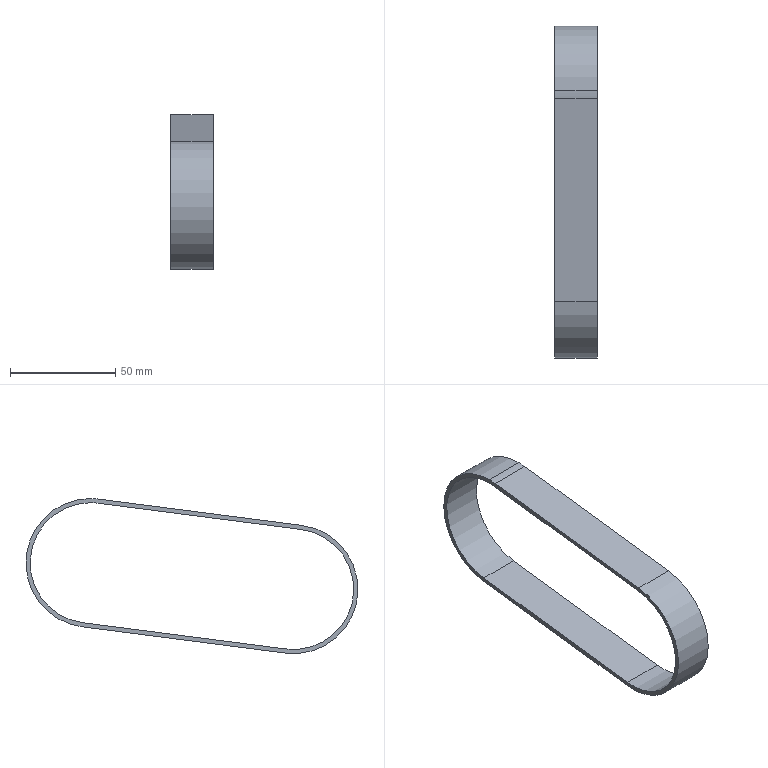Part | SolidWorks | features BaseBody 1 | 1 solid | 12 faces | box 20 x 157.99 x 73.8 mm | volume 15251 mm3 | cylinder 6 | plane 6 | commonest cylinder face diameters 57.3 x3 61.3 x3
STEP:
#1=CARTESIAN_POINT('',(20.,3.673,-28.414));
#2=VERTEX_POINT('',#1);
#3=CARTESIAN_POINT('',(20.,0.,28.65));
#4=VERTEX_POINT('',#3);
#5=CARTESIAN_POINT('',(20.,0.,0.));
#6=DIRECTION('',(1.,0.,0.));
#7=DIRECTION('',(0.,0.,-1.));
#8=AXIS2_PLACEMENT_3D('',#5,#6,#7);
#9=CIRCLE('',#8,28.65);
#10=EDGE_CURVE('',#2,#4,#9,.T.);
#11=ORIENTED_EDGE('',*,*,#10,.T.);
#12=CARTESIAN_POINT('',(0.,0.,28.65));
#13=VERTEX_POINT('',#12);
#14=CARTESIAN_POINT('',(20.,0.,28.65));
#15=DIRECTION('',(-1.,0.,0.));
#16=VECTOR('',#15,1000.);
#17=LINE('',#14,#16);
#18=EDGE_CURVE('',#4,#13,#17,.T.);
#19=ORIENTED_EDGE('',*,*,#18,.T.);
#20=CARTESIAN_POINT('',(0.,3.673,-28.414));
#21=VERTEX_POINT('',#20);
#22=CARTESIAN_POINT('',(0.,0.,0.));
#23=DIRECTION('',(1.,0.,0.));
#24=DIRECTION('',(0.,0.,-1.));
#25=AXIS2_PLACEMENT_3D('',#22,#23,#24);
#26=CIRCLE('',#25,28.65);
#27=EDGE_CURVE('',#21,#13,#26,.T.);
#28=ORIENTED_EDGE('',*,*,#27,.F.);
#29=CARTESIAN_POINT('',(20.,3.673,-28.414));
#30=DIRECTION('',(-1.,0.,0.));
#31=VECTOR('',#30,1000.);
#32=LINE('',#29,#31);
#33=EDGE_CURVE('',#2,#21,#32,.T.);
#34=ORIENTED_EDGE('',*,*,#33,.F.);
#35=EDGE_LOOP('',(#11,#19,#28,#34));
#36=FACE_OUTER_BOUND('',#35,.T.);
#37=CARTESIAN_POINT('',(20.,0.,0.));
#38=DIRECTION('',(-1.,0.,0.));
#39=DIRECTION('',(0.,0.,1.));
#40=AXIS2_PLACEMENT_3D('',#37,#38,#39);
#41=CYLINDRICAL_SURFACE('',#40,28.65);
#42=ADVANCED_FACE('',(#36),#41,.F.);
#43=CARTESIAN_POINT('',(20.,0.,30.65));
#44=VERTEX_POINT('',#43);
#45=CARTESIAN_POINT('',(20.,-3.93,30.397));
#46=VERTEX_POINT('',#45);
#47=CARTESIAN_POINT('',(20.,0.,0.));
#48=DIRECTION('',(1.,0.,0.));
#49=DIRECTION('',(0.,0.,-1.));
#50=AXIS2_PLACEMENT_3D('',#47,#48,#49);
#51=CIRCLE('',#50,30.65);
#52=EDGE_CURVE('',#44,#46,#51,.T.);
#53=ORIENTED_EDGE('',*,*,#52,.F.);
#54=CARTESIAN_POINT('',(0.,0.,30.65));
#55=VERTEX_POINT('',#54);
#56=CARTESIAN_POINT('',(20.,0.,30.65));
#57=DIRECTION('',(-1.,0.,0.));
#58=VECTOR('',#57,1000.);
#59=LINE('',#56,#58);
#60=EDGE_CURVE('',#44,#55,#59,.T.);
#61=ORIENTED_EDGE('',*,*,#60,.T.);
#62=CARTESIAN_POINT('',(0.,-3.93,30.397));
#63=VERTEX_POINT('',#62);
#64=CARTESIAN_POINT('',(0.,0.,0.));
#65=DIRECTION('',(1.,0.,0.));
#66=DIRECTION('',(0.,0.,-1.));
#67=AXIS2_PLACEMENT_3D('',#64,#65,#66);
#68=CIRCLE('',#67,30.65);
#69=EDGE_CURVE('',#55,#63,#68,.T.);
#70=ORIENTED_EDGE('',*,*,#69,.T.);
#71=CARTESIAN_POINT('',(20.,-3.93,30.397));
#72=DIRECTION('',(-1.,0.,0.));
#73=VECTOR('',#72,1000.);
#74=LINE('',#71,#73);
#75=EDGE_CURVE('',#46,#63,#74,.T.);
#76=ORIENTED_EDGE('',*,*,#75,.F.);
#77=EDGE_LOOP('',(#53,#61,#70,#76));
#78=FACE_OUTER_BOUND('',#77,.T.);
#79=CARTESIAN_POINT('',(20.,0.,0.));
#80=DIRECTION('',(-1.,0.,0.));
#81=DIRECTION('',(0.,0.,1.));
#82=AXIS2_PLACEMENT_3D('',#79,#80,#81);
#83=CYLINDRICAL_SURFACE('',#82,30.65);
#84=ADVANCED_FACE('',(#78),#83,.T.);
#85=CARTESIAN_POINT('',(0.,-93.017,-40.914));
#86=VERTEX_POINT('',#85);
#87=CARTESIAN_POINT('',(0.,3.673,-28.414));
#88=DIRECTION('',(0.,0.9917,0.1282));
#89=VECTOR('',#88,1000.);
#90=LINE('',#87,#89);
#91=EDGE_CURVE('',#86,#21,#90,.T.);
#92=ORIENTED_EDGE('',*,*,#91,.F.);
#93=CARTESIAN_POINT('',(20.,-93.017,-40.914));
#94=VERTEX_POINT('',#93);
#95=CARTESIAN_POINT('',(20.,-93.017,-40.914));
#96=DIRECTION('',(-1.,0.,0.));
#97=VECTOR('',#96,1000.);
#98=LINE('',#95,#97);
#99=EDGE_CURVE('',#94,#86,#98,.T.);
#100=ORIENTED_EDGE('',*,*,#99,.F.);
#101=CARTESIAN_POINT('',(20.,3.673,-28.414));
#102=DIRECTION('',(0.,0.9917,0.1282));
#103=VECTOR('',#102,1000.);
#104=LINE('',#101,#103);
#105=EDGE_CURVE('',#94,#2,#104,.T.);
#106=ORIENTED_EDGE('',*,*,#105,.T.);
#107=ORIENTED_EDGE('',*,*,#33,.T.);
#108=EDGE_LOOP('',(#92,#100,#106,#107));
#109=FACE_OUTER_BOUND('',#108,.T.);
#110=CARTESIAN_POINT('',(20.,3.673,-28.414));
#111=DIRECTION('',(0.,-0.1282,0.9917));
#112=DIRECTION('',(-1.,0.,0.));
#113=AXIS2_PLACEMENT_3D('',#110,#111,#112);
#114=PLANE('',#113);
#115=ADVANCED_FACE('',(#109),#114,.T.);
#116=CARTESIAN_POINT('',(0.,-100.363,15.914));
#117=VERTEX_POINT('',#116);
#118=CARTESIAN_POINT('',(0.,-96.69,-12.5));
#119=DIRECTION('',(1.,0.,0.));
#120=DIRECTION('',(0.,0.,-1.));
#121=AXIS2_PLACEMENT_3D('',#118,#119,#120);
#122=CIRCLE('',#121,28.65);
#123=EDGE_CURVE('',#117,#86,#122,.T.);
#124=ORIENTED_EDGE('',*,*,#123,.F.);
#125=CARTESIAN_POINT('',(20.,-100.363,15.914));
#126=VERTEX_POINT('',#125);
#127=CARTESIAN_POINT('',(20.,-100.363,15.914));
#128=DIRECTION('',(-1.,0.,0.));
#129=VECTOR('',#128,1000.);
#130=LINE('',#127,#129);
#131=EDGE_CURVE('',#126,#117,#130,.T.);
#132=ORIENTED_EDGE('',*,*,#131,.F.);
#133=CARTESIAN_POINT('',(20.,-96.69,-12.5));
#134=DIRECTION('',(1.,0.,0.));
#135=DIRECTION('',(0.,0.,-1.));
#136=AXIS2_PLACEMENT_3D('',#133,#134,#135);
#137=CIRCLE('',#136,28.65);
#138=EDGE_CURVE('',#126,#94,#137,.T.);
#139=ORIENTED_EDGE('',*,*,#138,.T.);
#140=ORIENTED_EDGE('',*,*,#99,.T.);
#141=EDGE_LOOP('',(#124,#132,#139,#140));
#142=FACE_OUTER_BOUND('',#141,.T.);
#143=CARTESIAN_POINT('',(20.,-96.69,-12.5));
#144=DIRECTION('',(-1.,0.,0.));
#145=DIRECTION('',(0.,0.,1.));
#146=AXIS2_PLACEMENT_3D('',#143,#144,#145);
#147=CYLINDRICAL_SURFACE('',#146,28.65);
#148=ADVANCED_FACE('',(#142),#147,.F.);
#149=CARTESIAN_POINT('',(0.,-3.673,28.414));
#150=VERTEX_POINT('',#149);
#151=CARTESIAN_POINT('',(0.,-3.673,28.414));
#152=DIRECTION('',(0.,-0.9917,-0.1282));
#153=VECTOR('',#152,1000.);
#154=LINE('',#151,#153);
#155=EDGE_CURVE('',#150,#117,#154,.T.);
#156=ORIENTED_EDGE('',*,*,#155,.F.);
#157=CARTESIAN_POINT('',(20.,-3.673,28.414));
#158=VERTEX_POINT('',#157);
#159=CARTESIAN_POINT('',(20.,-3.673,28.414));
#160=DIRECTION('',(-1.,0.,0.));
#161=VECTOR('',#160,1000.);
#162=LINE('',#159,#161);
#163=EDGE_CURVE('',#158,#150,#162,.T.);
#164=ORIENTED_EDGE('',*,*,#163,.F.);
#165=CARTESIAN_POINT('',(20.,-3.673,28.414));
#166=DIRECTION('',(0.,-0.9917,-0.1282));
#167=VECTOR('',#166,1000.);
#168=LINE('',#165,#167);
#169=EDGE_CURVE('',#158,#126,#168,.T.);
#170=ORIENTED_EDGE('',*,*,#169,.T.);
#171=ORIENTED_EDGE('',*,*,#131,.T.);
#172=EDGE_LOOP('',(#156,#164,#170,#171));
#173=FACE_OUTER_BOUND('',#172,.T.);
#174=CARTESIAN_POINT('',(20.,-3.673,28.414));
#175=DIRECTION('',(0.,0.1282,-0.9917));
#176=DIRECTION('',(-1.,0.,0.));
#177=AXIS2_PLACEMENT_3D('',#174,#175,#176);
#178=PLANE('',#177);
#179=ADVANCED_FACE('',(#173),#178,.T.);
#180=CARTESIAN_POINT('',(0.,-92.76,-42.897));
#181=VERTEX_POINT('',#180);
#182=CARTESIAN_POINT('',(0.,3.93,-30.397));
#183=VERTEX_POINT('',#182);
#184=CARTESIAN_POINT('',(0.,3.93,-30.397));
#185=DIRECTION('',(0.,0.9917,0.1282));
#186=VECTOR('',#185,1000.);
#187=LINE('',#184,#186);
#188=EDGE_CURVE('',#181,#183,#187,.T.);
#189=ORIENTED_EDGE('',*,*,#188,.T.);
#190=CARTESIAN_POINT('',(20.,3.93,-30.397));
#191=VERTEX_POINT('',#190);
#192=CARTESIAN_POINT('',(20.,3.93,-30.397));
#193=DIRECTION('',(-1.,0.,0.));
#194=VECTOR('',#193,1000.);
#195=LINE('',#192,#194);
#196=EDGE_CURVE('',#191,#183,#195,.T.);
#197=ORIENTED_EDGE('',*,*,#196,.F.);
#198=CARTESIAN_POINT('',(20.,-92.76,-42.897));
#199=VERTEX_POINT('',#198);
#200=CARTESIAN_POINT('',(20.,3.93,-30.397));
#201=DIRECTION('',(0.,0.9917,0.1282));
#202=VECTOR('',#201,1000.);
#203=LINE('',#200,#202);
#204=EDGE_CURVE('',#199,#191,#203,.T.);
#205=ORIENTED_EDGE('',*,*,#204,.F.);
#206=CARTESIAN_POINT('',(20.,-92.76,-42.897));
#207=DIRECTION('',(-1.,0.,0.));
#208=VECTOR('',#207,1000.);
#209=LINE('',#206,#208);
#210=EDGE_CURVE('',#199,#181,#209,.T.);
#211=ORIENTED_EDGE('',*,*,#210,.T.);
#212=EDGE_LOOP('',(#189,#197,#205,#211));
#213=FACE_OUTER_BOUND('',#212,.T.);
#214=CARTESIAN_POINT('',(20.,3.93,-30.397));
#215=DIRECTION('',(0.,-0.1282,0.9917));
#216=DIRECTION('',(-1.,0.,0.));
#217=AXIS2_PLACEMENT_3D('',#214,#215,#216);
#218=PLANE('',#217);
#219=ADVANCED_FACE('',(#213),#218,.F.);
#220=CARTESIAN_POINT('',(0.,-100.62,17.897));
#221=VERTEX_POINT('',#220);
#222=CARTESIAN_POINT('',(0.,-96.69,-12.5));
#223=DIRECTION('',(1.,0.,0.));
#224=DIRECTION('',(0.,0.,-1.));
#225=AXIS2_PLACEMENT_3D('',#222,#223,#224);
#226=CIRCLE('',#225,30.65);
#227=EDGE_CURVE('',#221,#181,#226,.T.);
#228=ORIENTED_EDGE('',*,*,#227,.T.);
#229=ORIENTED_EDGE('',*,*,#210,.F.);
#230=CARTESIAN_POINT('',(20.,-100.62,17.897));
#231=VERTEX_POINT('',#230);
#232=CARTESIAN_POINT('',(20.,-96.69,-12.5));
#233=DIRECTION('',(1.,0.,0.));
#234=DIRECTION('',(0.,0.,-1.));
#235=AXIS2_PLACEMENT_3D('',#232,#233,#234);
#236=CIRCLE('',#235,30.65);
#237=EDGE_CURVE('',#231,#199,#236,.T.);
#238=ORIENTED_EDGE('',*,*,#237,.F.);
#239=CARTESIAN_POINT('',(20.,-100.62,17.897));
#240=DIRECTION('',(-1.,0.,0.));
#241=VECTOR('',#240,1000.);
#242=LINE('',#239,#241);
#243=EDGE_CURVE('',#231,#221,#242,.T.);
#244=ORIENTED_EDGE('',*,*,#243,.T.);
#245=EDGE_LOOP('',(#228,#229,#238,#244));
#246=FACE_OUTER_BOUND('',#245,.T.);
#247=CARTESIAN_POINT('',(20.,-96.69,-12.5));
#248=DIRECTION('',(-1.,0.,0.));
#249=DIRECTION('',(0.,0.,1.));
#250=AXIS2_PLACEMENT_3D('',#247,#248,#249);
#251=CYLINDRICAL_SURFACE('',#250,30.65);
#252=ADVANCED_FACE('',(#246),#251,.T.);
#253=CARTESIAN_POINT('',(0.,-3.93,30.397));
#254=DIRECTION('',(0.,-0.9917,-0.1282));
#255=VECTOR('',#254,1000.);
#256=LINE('',#253,#255);
#257=EDGE_CURVE('',#63,#221,#256,.T.);
#258=ORIENTED_EDGE('',*,*,#257,.T.);
#259=ORIENTED_EDGE('',*,*,#243,.F.);
#260=CARTESIAN_POINT('',(20.,-3.93,30.397));
#261=DIRECTION('',(0.,-0.9917,-0.1282));
#262=VECTOR('',#261,1000.);
#263=LINE('',#260,#262);
#264=EDGE_CURVE('',#46,#231,#263,.T.);
#265=ORIENTED_EDGE('',*,*,#264,.F.);
#266=ORIENTED_EDGE('',*,*,#75,.T.);
#267=EDGE_LOOP('',(#258,#259,#265,#266));
#268=FACE_OUTER_BOUND('',#267,.T.);
#269=CARTESIAN_POINT('',(20.,-3.93,30.397));
#270=DIRECTION('',(0.,0.1282,-0.9917));
#271=DIRECTION('',(-1.,0.,0.));
#272=AXIS2_PLACEMENT_3D('',#269,#270,#271);
#273=PLANE('',#272);
#274=ADVANCED_FACE('',(#268),#273,.F.);
#275=ORIENTED_EDGE('',*,*,#27,.T.);
#276=CARTESIAN_POINT('',(0.,0.,0.));
#277=DIRECTION('',(1.,0.,0.));
#278=DIRECTION('',(0.,0.,-1.));
#279=AXIS2_PLACEMENT_3D('',#276,#277,#278);
#280=CIRCLE('',#279,28.65);
#281=EDGE_CURVE('',#13,#150,#280,.T.);
#282=ORIENTED_EDGE('',*,*,#281,.T.);
#283=ORIENTED_EDGE('',*,*,#155,.T.);
#284=ORIENTED_EDGE('',*,*,#123,.T.);
#285=ORIENTED_EDGE('',*,*,#91,.T.);
#286=EDGE_LOOP('',(#275,#282,#283,#284,#285));
#287=FACE_BOUND('',#286,.T.);
#288=CARTESIAN_POINT('',(0.,0.,0.));
#289=DIRECTION('',(1.,0.,0.));
#290=DIRECTION('',(0.,0.,-1.));
#291=AXIS2_PLACEMENT_3D('',#288,#289,#290);
#292=CIRCLE('',#291,30.65);
#293=EDGE_CURVE('',#183,#55,#292,.T.);
#294=ORIENTED_EDGE('',*,*,#293,.F.);
#295=ORIENTED_EDGE('',*,*,#188,.F.);
#296=ORIENTED_EDGE('',*,*,#227,.F.);
#297=ORIENTED_EDGE('',*,*,#257,.F.);
#298=ORIENTED_EDGE('',*,*,#69,.F.);
#299=EDGE_LOOP('',(#294,#295,#296,#297,#298));
#300=FACE_OUTER_BOUND('',#299,.T.);
#301=CARTESIAN_POINT('',(0.,0.,0.));
#302=DIRECTION('',(1.,0.,0.));
#303=DIRECTION('',(0.,1.,0.));
#304=AXIS2_PLACEMENT_3D('',#301,#302,#303);
#305=PLANE('',#304);
#306=ADVANCED_FACE('',(#287,#300),#305,.F.);
#307=ORIENTED_EDGE('',*,*,#169,.F.);
#308=CARTESIAN_POINT('',(20.,0.,0.));
#309=DIRECTION('',(1.,0.,0.));
#310=DIRECTION('',(0.,0.,-1.));
#311=AXIS2_PLACEMENT_3D('',#308,#309,#310);
#312=CIRCLE('',#311,28.65);
#313=EDGE_CURVE('',#4,#158,#312,.T.);
#314=ORIENTED_EDGE('',*,*,#313,.F.);
#315=ORIENTED_EDGE('',*,*,#10,.F.);
#316=ORIENTED_EDGE('',*,*,#105,.F.);
#317=ORIENTED_EDGE('',*,*,#138,.F.);
#318=EDGE_LOOP('',(#307,#314,#315,#316,#317));
#319=FACE_BOUND('',#318,.T.);
#320=ORIENTED_EDGE('',*,*,#204,.T.);
#321=CARTESIAN_POINT('',(20.,0.,0.));
#322=DIRECTION('',(1.,0.,0.));
#323=DIRECTION('',(0.,0.,-1.));
#324=AXIS2_PLACEMENT_3D('',#321,#322,#323);
#325=CIRCLE('',#324,30.65);
#326=EDGE_CURVE('',#191,#44,#325,.T.);
#327=ORIENTED_EDGE('',*,*,#326,.T.);
#328=ORIENTED_EDGE('',*,*,#52,.T.);
#329=ORIENTED_EDGE('',*,*,#264,.T.);
#330=ORIENTED_EDGE('',*,*,#237,.T.);
#331=EDGE_LOOP('',(#320,#327,#328,#329,#330));
#332=FACE_OUTER_BOUND('',#331,.T.);
#333=CARTESIAN_POINT('',(20.,0.,0.));
#334=DIRECTION('',(1.,0.,0.));
#335=DIRECTION('',(0.,1.,0.));
#336=AXIS2_PLACEMENT_3D('',#333,#334,#335);
#337=PLANE('',#336);
#338=ADVANCED_FACE('',(#319,#332),#337,.T.);
#339=ORIENTED_EDGE('',*,*,#60,.F.);
#340=ORIENTED_EDGE('',*,*,#326,.F.);
#341=ORIENTED_EDGE('',*,*,#196,.T.);
#342=ORIENTED_EDGE('',*,*,#293,.T.);
#343=EDGE_LOOP('',(#339,#340,#341,#342));
#344=FACE_OUTER_BOUND('',#343,.T.);
#345=CARTESIAN_POINT('',(20.,0.,0.));
#346=DIRECTION('',(-1.,0.,0.));
#347=DIRECTION('',(0.,0.,1.));
#348=AXIS2_PLACEMENT_3D('',#345,#346,#347);
#349=CYLINDRICAL_SURFACE('',#348,30.65);
#350=ADVANCED_FACE('',(#344),#349,.T.);
#351=ORIENTED_EDGE('',*,*,#18,.F.);
#352=ORIENTED_EDGE('',*,*,#313,.T.);
#353=ORIENTED_EDGE('',*,*,#163,.T.);
#354=ORIENTED_EDGE('',*,*,#281,.F.);
#355=EDGE_LOOP('',(#351,#352,#353,#354));
#356=FACE_OUTER_BOUND('',#355,.T.);
#357=CARTESIAN_POINT('',(20.,0.,0.));
#358=DIRECTION('',(-1.,0.,0.));
#359=DIRECTION('',(0.,0.,1.));
#360=AXIS2_PLACEMENT_3D('',#357,#358,#359);
#361=CYLINDRICAL_SURFACE('',#360,28.65);
#362=ADVANCED_FACE('',(#356),#361,.F.);
#363=CLOSED_SHELL('',(#42,#84,#115,#148,#179,#219,#252,#274,#306,#338,#350,#362));
#364=MANIFOLD_SOLID_BREP('',#363);
#365=CARTESIAN_POINT('',(0.,0.,0.));
#366=DIRECTION('',(0.,0.,1.));
#367=DIRECTION('',(1.,0.,0.));
#368=AXIS2_PLACEMENT_3D('',#365,#366,#367);
#369=(LENGTH_UNIT()NAMED_UNIT(*)SI_UNIT(.MILLI.,.METRE.));
#370=UNCERTAINTY_MEASURE_WITH_UNIT(LENGTH_MEASURE(0.00001),#369,'','');
#371=(NAMED_UNIT(*)PLANE_ANGLE_UNIT()SI_UNIT($,.RADIAN.));
#372=(NAMED_UNIT(*)SI_UNIT($,.STERADIAN.)SOLID_ANGLE_UNIT());
#373=(GEOMETRIC_REPRESENTATION_CONTEXT(3)GLOBAL_UNCERTAINTY_ASSIGNED_CONTEXT((#370))GLOBAL_UNIT_ASSIGNED_CONTEXT((#369,#371,#372))REPRESENTATION_CONTEXT('',''));
#374=ADVANCED_BREP_SHAPE_REPRESENTATION('',(#364,#368),#373);